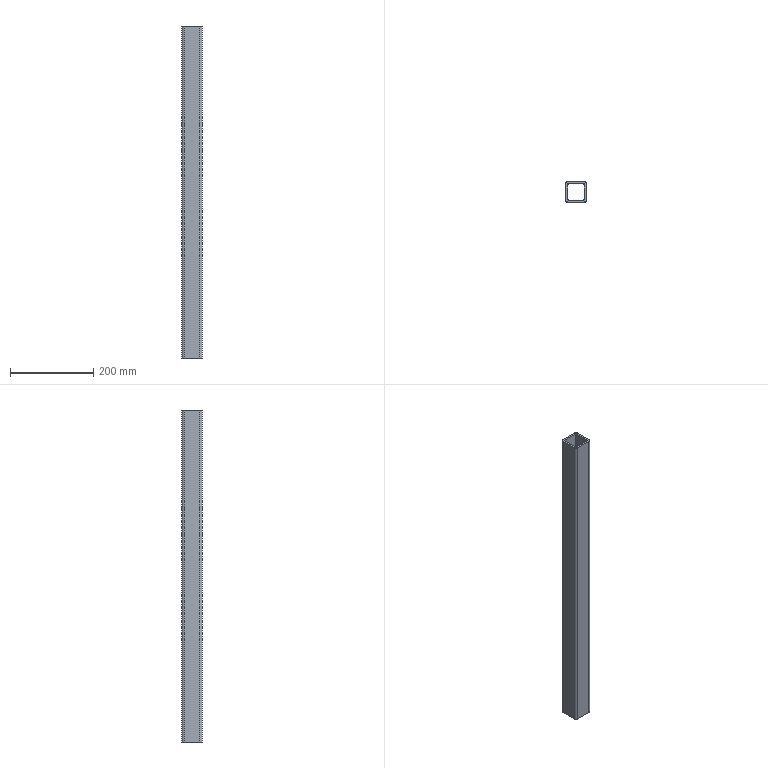Part | SolidWorks | features Extrusion 1 | 1 solid | 18 faces | box 50 x 50 x 800 mm | volume 695965 mm3 | plane 10 | cylinder 8 | commonest cylinder face diameters 2 x4 12 x4
STEP:
#1=CARTESIAN_POINT('',(0.,6.,800.));
#2=VERTEX_POINT('',#1);
#3=CARTESIAN_POINT('',(6.,0.,800.));
#4=VERTEX_POINT('',#3);
#5=CARTESIAN_POINT('',(6.,6.,800.));
#6=DIRECTION('',(0.,0.,1.));
#7=DIRECTION('',(-1.,0.,0.));
#8=AXIS2_PLACEMENT_3D('',#5,#6,#7);
#9=CIRCLE('',#8,6.);
#10=EDGE_CURVE('',#2,#4,#9,.T.);
#11=ORIENTED_EDGE('',*,*,#10,.T.);
#12=CARTESIAN_POINT('',(44.,0.,800.));
#13=VERTEX_POINT('',#12);
#14=CARTESIAN_POINT('',(6.,0.,800.));
#15=DIRECTION('',(1.,0.,0.));
#16=VECTOR('',#15,1000.);
#17=LINE('',#14,#16);
#18=EDGE_CURVE('',#4,#13,#17,.T.);
#19=ORIENTED_EDGE('',*,*,#18,.T.);
#20=CARTESIAN_POINT('',(50.,6.,800.));
#21=VERTEX_POINT('',#20);
#22=CARTESIAN_POINT('',(44.,6.,800.));
#23=DIRECTION('',(0.,0.,1.));
#24=DIRECTION('',(1.,0.,0.));
#25=AXIS2_PLACEMENT_3D('',#22,#23,#24);
#26=CIRCLE('',#25,6.);
#27=EDGE_CURVE('',#13,#21,#26,.T.);
#28=ORIENTED_EDGE('',*,*,#27,.T.);
#29=CARTESIAN_POINT('',(50.,44.,800.));
#30=VERTEX_POINT('',#29);
#31=CARTESIAN_POINT('',(50.,6.,800.));
#32=DIRECTION('',(0.,1.,0.));
#33=VECTOR('',#32,1000.);
#34=LINE('',#31,#33);
#35=EDGE_CURVE('',#21,#30,#34,.T.);
#36=ORIENTED_EDGE('',*,*,#35,.T.);
#37=CARTESIAN_POINT('',(44.,50.,800.));
#38=VERTEX_POINT('',#37);
#39=CARTESIAN_POINT('',(44.,44.,800.));
#40=DIRECTION('',(0.,0.,1.));
#41=DIRECTION('',(-1.,0.,0.));
#42=AXIS2_PLACEMENT_3D('',#39,#40,#41);
#43=CIRCLE('',#42,6.);
#44=EDGE_CURVE('',#30,#38,#43,.T.);
#45=ORIENTED_EDGE('',*,*,#44,.T.);
#46=CARTESIAN_POINT('',(6.,50.,800.));
#47=VERTEX_POINT('',#46);
#48=CARTESIAN_POINT('',(6.,50.,800.));
#49=DIRECTION('',(-1.,0.,0.));
#50=VECTOR('',#49,1000.);
#51=LINE('',#48,#50);
#52=EDGE_CURVE('',#38,#47,#51,.T.);
#53=ORIENTED_EDGE('',*,*,#52,.T.);
#54=CARTESIAN_POINT('',(0.,44.,800.));
#55=VERTEX_POINT('',#54);
#56=CARTESIAN_POINT('',(6.,44.,800.));
#57=DIRECTION('',(0.,0.,1.));
#58=DIRECTION('',(-1.,0.,0.));
#59=AXIS2_PLACEMENT_3D('',#56,#57,#58);
#60=CIRCLE('',#59,6.);
#61=EDGE_CURVE('',#47,#55,#60,.T.);
#62=ORIENTED_EDGE('',*,*,#61,.T.);
#63=CARTESIAN_POINT('',(0.,6.,800.));
#64=DIRECTION('',(0.,-1.,0.));
#65=VECTOR('',#64,1000.);
#66=LINE('',#63,#65);
#67=EDGE_CURVE('',#55,#2,#66,.T.);
#68=ORIENTED_EDGE('',*,*,#67,.T.);
#69=EDGE_LOOP('',(#11,#19,#28,#36,#45,#53,#62,#68));
#70=FACE_OUTER_BOUND('',#69,.T.);
#71=CARTESIAN_POINT('',(6.,45.,800.));
#72=VERTEX_POINT('',#71);
#73=CARTESIAN_POINT('',(5.,44.,800.));
#74=VERTEX_POINT('',#73);
#75=CARTESIAN_POINT('',(6.,44.,800.));
#76=DIRECTION('',(0.,0.,1.));
#77=DIRECTION('',(-1.,0.,0.));
#78=AXIS2_PLACEMENT_3D('',#75,#76,#77);
#79=CIRCLE('',#78,1.);
#80=EDGE_CURVE('',#72,#74,#79,.T.);
#81=ORIENTED_EDGE('',*,*,#80,.F.);
#82=CARTESIAN_POINT('',(44.,45.,800.));
#83=VERTEX_POINT('',#82);
#84=CARTESIAN_POINT('',(6.,45.,800.));
#85=DIRECTION('',(-1.,0.,0.));
#86=VECTOR('',#85,1000.);
#87=LINE('',#84,#86);
#88=EDGE_CURVE('',#83,#72,#87,.T.);
#89=ORIENTED_EDGE('',*,*,#88,.F.);
#90=CARTESIAN_POINT('',(45.,44.,800.));
#91=VERTEX_POINT('',#90);
#92=CARTESIAN_POINT('',(44.,44.,800.));
#93=DIRECTION('',(0.,0.,1.));
#94=DIRECTION('',(-1.,0.,0.));
#95=AXIS2_PLACEMENT_3D('',#92,#93,#94);
#96=CIRCLE('',#95,1.);
#97=EDGE_CURVE('',#91,#83,#96,.T.);
#98=ORIENTED_EDGE('',*,*,#97,.F.);
#99=CARTESIAN_POINT('',(45.,6.,800.));
#100=VERTEX_POINT('',#99);
#101=CARTESIAN_POINT('',(45.,6.,800.));
#102=DIRECTION('',(0.,1.,0.));
#103=VECTOR('',#102,1000.);
#104=LINE('',#101,#103);
#105=EDGE_CURVE('',#100,#91,#104,.T.);
#106=ORIENTED_EDGE('',*,*,#105,.F.);
#107=CARTESIAN_POINT('',(44.,5.,800.));
#108=VERTEX_POINT('',#107);
#109=CARTESIAN_POINT('',(44.,6.,800.));
#110=DIRECTION('',(0.,0.,1.));
#111=DIRECTION('',(1.,0.,0.));
#112=AXIS2_PLACEMENT_3D('',#109,#110,#111);
#113=CIRCLE('',#112,1.);
#114=EDGE_CURVE('',#108,#100,#113,.T.);
#115=ORIENTED_EDGE('',*,*,#114,.F.);
#116=CARTESIAN_POINT('',(6.,5.,800.));
#117=VERTEX_POINT('',#116);
#118=CARTESIAN_POINT('',(6.,5.,800.));
#119=DIRECTION('',(1.,0.,0.));
#120=VECTOR('',#119,1000.);
#121=LINE('',#118,#120);
#122=EDGE_CURVE('',#117,#108,#121,.T.);
#123=ORIENTED_EDGE('',*,*,#122,.F.);
#124=CARTESIAN_POINT('',(5.,6.,800.));
#125=VERTEX_POINT('',#124);
#126=CARTESIAN_POINT('',(6.,6.,800.));
#127=DIRECTION('',(0.,0.,1.));
#128=DIRECTION('',(-1.,0.,0.));
#129=AXIS2_PLACEMENT_3D('',#126,#127,#128);
#130=CIRCLE('',#129,1.);
#131=EDGE_CURVE('',#125,#117,#130,.T.);
#132=ORIENTED_EDGE('',*,*,#131,.F.);
#133=CARTESIAN_POINT('',(5.,6.,800.));
#134=DIRECTION('',(0.,-1.,0.));
#135=VECTOR('',#134,1000.);
#136=LINE('',#133,#135);
#137=EDGE_CURVE('',#74,#125,#136,.T.);
#138=ORIENTED_EDGE('',*,*,#137,.F.);
#139=EDGE_LOOP('',(#81,#89,#98,#106,#115,#123,#132,#138));
#140=FACE_BOUND('',#139,.T.);
#141=CARTESIAN_POINT('',(6.,6.,800.));
#142=DIRECTION('',(0.,0.,-1.));
#143=DIRECTION('',(-1.,0.,0.));
#144=AXIS2_PLACEMENT_3D('',#141,#142,#143);
#145=PLANE('',#144);
#146=ADVANCED_FACE('',(#70,#140),#145,.F.);
#147=CARTESIAN_POINT('',(0.,6.,0.));
#148=VERTEX_POINT('',#147);
#149=CARTESIAN_POINT('',(6.,0.,0.));
#150=VERTEX_POINT('',#149);
#151=CARTESIAN_POINT('',(6.,6.,0.));
#152=DIRECTION('',(0.,0.,1.));
#153=DIRECTION('',(-1.,0.,0.));
#154=AXIS2_PLACEMENT_3D('',#151,#152,#153);
#155=CIRCLE('',#154,6.);
#156=EDGE_CURVE('',#148,#150,#155,.T.);
#157=ORIENTED_EDGE('',*,*,#156,.F.);
#158=CARTESIAN_POINT('',(0.,44.,0.));
#159=VERTEX_POINT('',#158);
#160=CARTESIAN_POINT('',(0.,6.,0.));
#161=DIRECTION('',(0.,-1.,0.));
#162=VECTOR('',#161,1000.);
#163=LINE('',#160,#162);
#164=EDGE_CURVE('',#159,#148,#163,.T.);
#165=ORIENTED_EDGE('',*,*,#164,.F.);
#166=CARTESIAN_POINT('',(6.,50.,0.));
#167=VERTEX_POINT('',#166);
#168=CARTESIAN_POINT('',(6.,44.,0.));
#169=DIRECTION('',(0.,0.,1.));
#170=DIRECTION('',(-1.,0.,0.));
#171=AXIS2_PLACEMENT_3D('',#168,#169,#170);
#172=CIRCLE('',#171,6.);
#173=EDGE_CURVE('',#167,#159,#172,.T.);
#174=ORIENTED_EDGE('',*,*,#173,.F.);
#175=CARTESIAN_POINT('',(44.,50.,0.));
#176=VERTEX_POINT('',#175);
#177=CARTESIAN_POINT('',(6.,50.,0.));
#178=DIRECTION('',(-1.,0.,0.));
#179=VECTOR('',#178,1000.);
#180=LINE('',#177,#179);
#181=EDGE_CURVE('',#176,#167,#180,.T.);
#182=ORIENTED_EDGE('',*,*,#181,.F.);
#183=CARTESIAN_POINT('',(50.,44.,0.));
#184=VERTEX_POINT('',#183);
#185=CARTESIAN_POINT('',(44.,44.,0.));
#186=DIRECTION('',(0.,0.,1.));
#187=DIRECTION('',(-1.,0.,0.));
#188=AXIS2_PLACEMENT_3D('',#185,#186,#187);
#189=CIRCLE('',#188,6.);
#190=EDGE_CURVE('',#184,#176,#189,.T.);
#191=ORIENTED_EDGE('',*,*,#190,.F.);
#192=CARTESIAN_POINT('',(50.,6.,0.));
#193=VERTEX_POINT('',#192);
#194=CARTESIAN_POINT('',(50.,6.,0.));
#195=DIRECTION('',(0.,1.,0.));
#196=VECTOR('',#195,1000.);
#197=LINE('',#194,#196);
#198=EDGE_CURVE('',#193,#184,#197,.T.);
#199=ORIENTED_EDGE('',*,*,#198,.F.);
#200=CARTESIAN_POINT('',(44.,0.,0.));
#201=VERTEX_POINT('',#200);
#202=CARTESIAN_POINT('',(44.,6.,0.));
#203=DIRECTION('',(0.,0.,1.));
#204=DIRECTION('',(1.,0.,0.));
#205=AXIS2_PLACEMENT_3D('',#202,#203,#204);
#206=CIRCLE('',#205,6.);
#207=EDGE_CURVE('',#201,#193,#206,.T.);
#208=ORIENTED_EDGE('',*,*,#207,.F.);
#209=CARTESIAN_POINT('',(6.,0.,0.));
#210=DIRECTION('',(1.,0.,0.));
#211=VECTOR('',#210,1000.);
#212=LINE('',#209,#211);
#213=EDGE_CURVE('',#150,#201,#212,.T.);
#214=ORIENTED_EDGE('',*,*,#213,.F.);
#215=EDGE_LOOP('',(#157,#165,#174,#182,#191,#199,#208,#214));
#216=FACE_OUTER_BOUND('',#215,.T.);
#217=CARTESIAN_POINT('',(44.,45.,0.));
#218=VERTEX_POINT('',#217);
#219=CARTESIAN_POINT('',(6.,45.,0.));
#220=VERTEX_POINT('',#219);
#221=CARTESIAN_POINT('',(6.,45.,0.));
#222=DIRECTION('',(-1.,0.,0.));
#223=VECTOR('',#222,1000.);
#224=LINE('',#221,#223);
#225=EDGE_CURVE('',#218,#220,#224,.T.);
#226=ORIENTED_EDGE('',*,*,#225,.T.);
#227=CARTESIAN_POINT('',(5.,44.,0.));
#228=VERTEX_POINT('',#227);
#229=CARTESIAN_POINT('',(6.,44.,0.));
#230=DIRECTION('',(0.,0.,1.));
#231=DIRECTION('',(-1.,0.,0.));
#232=AXIS2_PLACEMENT_3D('',#229,#230,#231);
#233=CIRCLE('',#232,1.);
#234=EDGE_CURVE('',#220,#228,#233,.T.);
#235=ORIENTED_EDGE('',*,*,#234,.T.);
#236=CARTESIAN_POINT('',(5.,6.,0.));
#237=VERTEX_POINT('',#236);
#238=CARTESIAN_POINT('',(5.,6.,0.));
#239=DIRECTION('',(0.,-1.,0.));
#240=VECTOR('',#239,1000.);
#241=LINE('',#238,#240);
#242=EDGE_CURVE('',#228,#237,#241,.T.);
#243=ORIENTED_EDGE('',*,*,#242,.T.);
#244=CARTESIAN_POINT('',(6.,5.,0.));
#245=VERTEX_POINT('',#244);
#246=CARTESIAN_POINT('',(6.,6.,0.));
#247=DIRECTION('',(0.,0.,1.));
#248=DIRECTION('',(-1.,0.,0.));
#249=AXIS2_PLACEMENT_3D('',#246,#247,#248);
#250=CIRCLE('',#249,1.);
#251=EDGE_CURVE('',#237,#245,#250,.T.);
#252=ORIENTED_EDGE('',*,*,#251,.T.);
#253=CARTESIAN_POINT('',(44.,5.,0.));
#254=VERTEX_POINT('',#253);
#255=CARTESIAN_POINT('',(6.,5.,0.));
#256=DIRECTION('',(1.,0.,0.));
#257=VECTOR('',#256,1000.);
#258=LINE('',#255,#257);
#259=EDGE_CURVE('',#245,#254,#258,.T.);
#260=ORIENTED_EDGE('',*,*,#259,.T.);
#261=CARTESIAN_POINT('',(45.,6.,0.));
#262=VERTEX_POINT('',#261);
#263=CARTESIAN_POINT('',(44.,6.,0.));
#264=DIRECTION('',(0.,0.,1.));
#265=DIRECTION('',(1.,0.,0.));
#266=AXIS2_PLACEMENT_3D('',#263,#264,#265);
#267=CIRCLE('',#266,1.);
#268=EDGE_CURVE('',#254,#262,#267,.T.);
#269=ORIENTED_EDGE('',*,*,#268,.T.);
#270=CARTESIAN_POINT('',(45.,44.,0.));
#271=VERTEX_POINT('',#270);
#272=CARTESIAN_POINT('',(45.,6.,0.));
#273=DIRECTION('',(0.,1.,0.));
#274=VECTOR('',#273,1000.);
#275=LINE('',#272,#274);
#276=EDGE_CURVE('',#262,#271,#275,.T.);
#277=ORIENTED_EDGE('',*,*,#276,.T.);
#278=CARTESIAN_POINT('',(44.,44.,0.));
#279=DIRECTION('',(0.,0.,1.));
#280=DIRECTION('',(-1.,0.,0.));
#281=AXIS2_PLACEMENT_3D('',#278,#279,#280);
#282=CIRCLE('',#281,1.);
#283=EDGE_CURVE('',#271,#218,#282,.T.);
#284=ORIENTED_EDGE('',*,*,#283,.T.);
#285=EDGE_LOOP('',(#226,#235,#243,#252,#260,#269,#277,#284));
#286=FACE_BOUND('',#285,.T.);
#287=CARTESIAN_POINT('',(6.,6.,0.));
#288=DIRECTION('',(0.,0.,-1.));
#289=DIRECTION('',(-1.,0.,0.));
#290=AXIS2_PLACEMENT_3D('',#287,#288,#289);
#291=PLANE('',#290);
#292=ADVANCED_FACE('',(#216,#286),#291,.T.);
#293=ORIENTED_EDGE('',*,*,#156,.T.);
#294=CARTESIAN_POINT('',(6.,0.,800.));
#295=DIRECTION('',(0.,0.,-1.));
#296=VECTOR('',#295,1000.);
#297=LINE('',#294,#296);
#298=EDGE_CURVE('',#4,#150,#297,.T.);
#299=ORIENTED_EDGE('',*,*,#298,.F.);
#300=ORIENTED_EDGE('',*,*,#10,.F.);
#301=CARTESIAN_POINT('',(0.,6.,800.));
#302=DIRECTION('',(0.,0.,-1.));
#303=VECTOR('',#302,1000.);
#304=LINE('',#301,#303);
#305=EDGE_CURVE('',#2,#148,#304,.T.);
#306=ORIENTED_EDGE('',*,*,#305,.T.);
#307=EDGE_LOOP('',(#293,#299,#300,#306));
#308=FACE_OUTER_BOUND('',#307,.T.);
#309=CARTESIAN_POINT('',(6.,6.,800.));
#310=DIRECTION('',(0.,0.,-1.));
#311=DIRECTION('',(-1.,0.,0.));
#312=AXIS2_PLACEMENT_3D('',#309,#310,#311);
#313=CYLINDRICAL_SURFACE('',#312,6.);
#314=ADVANCED_FACE('',(#308),#313,.T.);
#315=ORIENTED_EDGE('',*,*,#213,.T.);
#316=CARTESIAN_POINT('',(44.,0.,800.));
#317=DIRECTION('',(0.,0.,-1.));
#318=VECTOR('',#317,1000.);
#319=LINE('',#316,#318);
#320=EDGE_CURVE('',#13,#201,#319,.T.);
#321=ORIENTED_EDGE('',*,*,#320,.F.);
#322=ORIENTED_EDGE('',*,*,#18,.F.);
#323=ORIENTED_EDGE('',*,*,#298,.T.);
#324=EDGE_LOOP('',(#315,#321,#322,#323));
#325=FACE_OUTER_BOUND('',#324,.T.);
#326=CARTESIAN_POINT('',(6.,0.,800.));
#327=DIRECTION('',(0.,1.,0.));
#328=DIRECTION('',(0.,0.,1.));
#329=AXIS2_PLACEMENT_3D('',#326,#327,#328);
#330=PLANE('',#329);
#331=ADVANCED_FACE('',(#325),#330,.F.);
#332=ORIENTED_EDGE('',*,*,#207,.T.);
#333=CARTESIAN_POINT('',(50.,6.,800.));
#334=DIRECTION('',(0.,0.,-1.));
#335=VECTOR('',#334,1000.);
#336=LINE('',#333,#335);
#337=EDGE_CURVE('',#21,#193,#336,.T.);
#338=ORIENTED_EDGE('',*,*,#337,.F.);
#339=ORIENTED_EDGE('',*,*,#27,.F.);
#340=ORIENTED_EDGE('',*,*,#320,.T.);
#341=EDGE_LOOP('',(#332,#338,#339,#340));
#342=FACE_OUTER_BOUND('',#341,.T.);
#343=CARTESIAN_POINT('',(44.,6.,800.));
#344=DIRECTION('',(0.,0.,-1.));
#345=DIRECTION('',(-1.,0.,0.));
#346=AXIS2_PLACEMENT_3D('',#343,#344,#345);
#347=CYLINDRICAL_SURFACE('',#346,6.);
#348=ADVANCED_FACE('',(#342),#347,.T.);
#349=ORIENTED_EDGE('',*,*,#198,.T.);
#350=CARTESIAN_POINT('',(50.,44.,800.));
#351=DIRECTION('',(0.,0.,-1.));
#352=VECTOR('',#351,1000.);
#353=LINE('',#350,#352);
#354=EDGE_CURVE('',#30,#184,#353,.T.);
#355=ORIENTED_EDGE('',*,*,#354,.F.);
#356=ORIENTED_EDGE('',*,*,#35,.F.);
#357=ORIENTED_EDGE('',*,*,#337,.T.);
#358=EDGE_LOOP('',(#349,#355,#356,#357));
#359=FACE_OUTER_BOUND('',#358,.T.);
#360=CARTESIAN_POINT('',(50.,6.,800.));
#361=DIRECTION('',(-1.,0.,0.));
#362=DIRECTION('',(0.,0.,1.));
#363=AXIS2_PLACEMENT_3D('',#360,#361,#362);
#364=PLANE('',#363);
#365=ADVANCED_FACE('',(#359),#364,.F.);
#366=ORIENTED_EDGE('',*,*,#190,.T.);
#367=CARTESIAN_POINT('',(44.,50.,800.));
#368=DIRECTION('',(0.,0.,-1.));
#369=VECTOR('',#368,1000.);
#370=LINE('',#367,#369);
#371=EDGE_CURVE('',#38,#176,#370,.T.);
#372=ORIENTED_EDGE('',*,*,#371,.F.);
#373=ORIENTED_EDGE('',*,*,#44,.F.);
#374=ORIENTED_EDGE('',*,*,#354,.T.);
#375=EDGE_LOOP('',(#366,#372,#373,#374));
#376=FACE_OUTER_BOUND('',#375,.T.);
#377=CARTESIAN_POINT('',(44.,44.,800.));
#378=DIRECTION('',(0.,0.,-1.));
#379=DIRECTION('',(-1.,0.,0.));
#380=AXIS2_PLACEMENT_3D('',#377,#378,#379);
#381=CYLINDRICAL_SURFACE('',#380,6.);
#382=ADVANCED_FACE('',(#376),#381,.T.);
#383=ORIENTED_EDGE('',*,*,#181,.T.);
#384=CARTESIAN_POINT('',(6.,50.,800.));
#385=DIRECTION('',(0.,0.,-1.));
#386=VECTOR('',#385,1000.);
#387=LINE('',#384,#386);
#388=EDGE_CURVE('',#47,#167,#387,.T.);
#389=ORIENTED_EDGE('',*,*,#388,.F.);
#390=ORIENTED_EDGE('',*,*,#52,.F.);
#391=ORIENTED_EDGE('',*,*,#371,.T.);
#392=EDGE_LOOP('',(#383,#389,#390,#391));
#393=FACE_OUTER_BOUND('',#392,.T.);
#394=CARTESIAN_POINT('',(6.,50.,800.));
#395=DIRECTION('',(0.,-1.,0.));
#396=DIRECTION('',(0.,0.,-1.));
#397=AXIS2_PLACEMENT_3D('',#394,#395,#396);
#398=PLANE('',#397);
#399=ADVANCED_FACE('',(#393),#398,.F.);
#400=ORIENTED_EDGE('',*,*,#173,.T.);
#401=CARTESIAN_POINT('',(0.,44.,800.));
#402=DIRECTION('',(0.,0.,-1.));
#403=VECTOR('',#402,1000.);
#404=LINE('',#401,#403);
#405=EDGE_CURVE('',#55,#159,#404,.T.);
#406=ORIENTED_EDGE('',*,*,#405,.F.);
#407=ORIENTED_EDGE('',*,*,#61,.F.);
#408=ORIENTED_EDGE('',*,*,#388,.T.);
#409=EDGE_LOOP('',(#400,#406,#407,#408));
#410=FACE_OUTER_BOUND('',#409,.T.);
#411=CARTESIAN_POINT('',(6.,44.,800.));
#412=DIRECTION('',(0.,0.,-1.));
#413=DIRECTION('',(-1.,0.,0.));
#414=AXIS2_PLACEMENT_3D('',#411,#412,#413);
#415=CYLINDRICAL_SURFACE('',#414,6.);
#416=ADVANCED_FACE('',(#410),#415,.T.);
#417=ORIENTED_EDGE('',*,*,#164,.T.);
#418=ORIENTED_EDGE('',*,*,#305,.F.);
#419=ORIENTED_EDGE('',*,*,#67,.F.);
#420=ORIENTED_EDGE('',*,*,#405,.T.);
#421=EDGE_LOOP('',(#417,#418,#419,#420));
#422=FACE_OUTER_BOUND('',#421,.T.);
#423=CARTESIAN_POINT('',(0.,6.,800.));
#424=DIRECTION('',(1.,0.,0.));
#425=DIRECTION('',(0.,0.,-1.));
#426=AXIS2_PLACEMENT_3D('',#423,#424,#425);
#427=PLANE('',#426);
#428=ADVANCED_FACE('',(#422),#427,.F.);
#429=ORIENTED_EDGE('',*,*,#234,.F.);
#430=CARTESIAN_POINT('',(6.,45.,800.));
#431=DIRECTION('',(0.,0.,-1.));
#432=VECTOR('',#431,1000.);
#433=LINE('',#430,#432);
#434=EDGE_CURVE('',#72,#220,#433,.T.);
#435=ORIENTED_EDGE('',*,*,#434,.F.);
#436=ORIENTED_EDGE('',*,*,#80,.T.);
#437=CARTESIAN_POINT('',(5.,44.,800.));
#438=DIRECTION('',(0.,0.,-1.));
#439=VECTOR('',#438,1000.);
#440=LINE('',#437,#439);
#441=EDGE_CURVE('',#74,#228,#440,.T.);
#442=ORIENTED_EDGE('',*,*,#441,.T.);
#443=EDGE_LOOP('',(#429,#435,#436,#442));
#444=FACE_OUTER_BOUND('',#443,.T.);
#445=CARTESIAN_POINT('',(6.,44.,800.));
#446=DIRECTION('',(0.,0.,-1.));
#447=DIRECTION('',(-1.,0.,0.));
#448=AXIS2_PLACEMENT_3D('',#445,#446,#447);
#449=CYLINDRICAL_SURFACE('',#448,1.);
#450=ADVANCED_FACE('',(#444),#449,.F.);
#451=ORIENTED_EDGE('',*,*,#242,.F.);
#452=ORIENTED_EDGE('',*,*,#441,.F.);
#453=ORIENTED_EDGE('',*,*,#137,.T.);
#454=CARTESIAN_POINT('',(5.,6.,800.));
#455=DIRECTION('',(0.,0.,-1.));
#456=VECTOR('',#455,1000.);
#457=LINE('',#454,#456);
#458=EDGE_CURVE('',#125,#237,#457,.T.);
#459=ORIENTED_EDGE('',*,*,#458,.T.);
#460=EDGE_LOOP('',(#451,#452,#453,#459));
#461=FACE_OUTER_BOUND('',#460,.T.);
#462=CARTESIAN_POINT('',(5.,6.,800.));
#463=DIRECTION('',(1.,0.,0.));
#464=DIRECTION('',(0.,1.,0.));
#465=AXIS2_PLACEMENT_3D('',#462,#463,#464);
#466=PLANE('',#465);
#467=ADVANCED_FACE('',(#461),#466,.T.);
#468=ORIENTED_EDGE('',*,*,#251,.F.);
#469=ORIENTED_EDGE('',*,*,#458,.F.);
#470=ORIENTED_EDGE('',*,*,#131,.T.);
#471=CARTESIAN_POINT('',(6.,5.,800.));
#472=DIRECTION('',(0.,0.,-1.));
#473=VECTOR('',#472,1000.);
#474=LINE('',#471,#473);
#475=EDGE_CURVE('',#117,#245,#474,.T.);
#476=ORIENTED_EDGE('',*,*,#475,.T.);
#477=EDGE_LOOP('',(#468,#469,#470,#476));
#478=FACE_OUTER_BOUND('',#477,.T.);
#479=CARTESIAN_POINT('',(6.,6.,800.));
#480=DIRECTION('',(0.,0.,-1.));
#481=DIRECTION('',(-1.,0.,0.));
#482=AXIS2_PLACEMENT_3D('',#479,#480,#481);
#483=CYLINDRICAL_SURFACE('',#482,1.);
#484=ADVANCED_FACE('',(#478),#483,.F.);
#485=ORIENTED_EDGE('',*,*,#259,.F.);
#486=ORIENTED_EDGE('',*,*,#475,.F.);
#487=ORIENTED_EDGE('',*,*,#122,.T.);
#488=CARTESIAN_POINT('',(44.,5.,800.));
#489=DIRECTION('',(0.,0.,-1.));
#490=VECTOR('',#489,1000.);
#491=LINE('',#488,#490);
#492=EDGE_CURVE('',#108,#254,#491,.T.);
#493=ORIENTED_EDGE('',*,*,#492,.T.);
#494=EDGE_LOOP('',(#485,#486,#487,#493));
#495=FACE_OUTER_BOUND('',#494,.T.);
#496=CARTESIAN_POINT('',(6.,5.,800.));
#497=DIRECTION('',(0.,1.,0.));
#498=DIRECTION('',(-1.,0.,0.));
#499=AXIS2_PLACEMENT_3D('',#496,#497,#498);
#500=PLANE('',#499);
#501=ADVANCED_FACE('',(#495),#500,.T.);
#502=ORIENTED_EDGE('',*,*,#268,.F.);
#503=ORIENTED_EDGE('',*,*,#492,.F.);
#504=ORIENTED_EDGE('',*,*,#114,.T.);
#505=CARTESIAN_POINT('',(45.,6.,800.));
#506=DIRECTION('',(0.,0.,-1.));
#507=VECTOR('',#506,1000.);
#508=LINE('',#505,#507);
#509=EDGE_CURVE('',#100,#262,#508,.T.);
#510=ORIENTED_EDGE('',*,*,#509,.T.);
#511=EDGE_LOOP('',(#502,#503,#504,#510));
#512=FACE_OUTER_BOUND('',#511,.T.);
#513=CARTESIAN_POINT('',(44.,6.,800.));
#514=DIRECTION('',(0.,0.,-1.));
#515=DIRECTION('',(-1.,0.,0.));
#516=AXIS2_PLACEMENT_3D('',#513,#514,#515);
#517=CYLINDRICAL_SURFACE('',#516,1.);
#518=ADVANCED_FACE('',(#512),#517,.F.);
#519=ORIENTED_EDGE('',*,*,#276,.F.);
#520=ORIENTED_EDGE('',*,*,#509,.F.);
#521=ORIENTED_EDGE('',*,*,#105,.T.);
#522=CARTESIAN_POINT('',(45.,44.,800.));
#523=DIRECTION('',(0.,0.,-1.));
#524=VECTOR('',#523,1000.);
#525=LINE('',#522,#524);
#526=EDGE_CURVE('',#91,#271,#525,.T.);
#527=ORIENTED_EDGE('',*,*,#526,.T.);
#528=EDGE_LOOP('',(#519,#520,#521,#527));
#529=FACE_OUTER_BOUND('',#528,.T.);
#530=CARTESIAN_POINT('',(45.,6.,800.));
#531=DIRECTION('',(-1.,0.,0.));
#532=DIRECTION('',(0.,0.,1.));
#533=AXIS2_PLACEMENT_3D('',#530,#531,#532);
#534=PLANE('',#533);
#535=ADVANCED_FACE('',(#529),#534,.T.);
#536=ORIENTED_EDGE('',*,*,#283,.F.);
#537=ORIENTED_EDGE('',*,*,#526,.F.);
#538=ORIENTED_EDGE('',*,*,#97,.T.);
#539=CARTESIAN_POINT('',(44.,45.,800.));
#540=DIRECTION('',(0.,0.,-1.));
#541=VECTOR('',#540,1000.);
#542=LINE('',#539,#541);
#543=EDGE_CURVE('',#83,#218,#542,.T.);
#544=ORIENTED_EDGE('',*,*,#543,.T.);
#545=EDGE_LOOP('',(#536,#537,#538,#544));
#546=FACE_OUTER_BOUND('',#545,.T.);
#547=CARTESIAN_POINT('',(44.,44.,800.));
#548=DIRECTION('',(0.,0.,-1.));
#549=DIRECTION('',(-1.,0.,0.));
#550=AXIS2_PLACEMENT_3D('',#547,#548,#549);
#551=CYLINDRICAL_SURFACE('',#550,1.);
#552=ADVANCED_FACE('',(#546),#551,.F.);
#553=ORIENTED_EDGE('',*,*,#225,.F.);
#554=ORIENTED_EDGE('',*,*,#543,.F.);
#555=ORIENTED_EDGE('',*,*,#88,.T.);
#556=ORIENTED_EDGE('',*,*,#434,.T.);
#557=EDGE_LOOP('',(#553,#554,#555,#556));
#558=FACE_OUTER_BOUND('',#557,.T.);
#559=CARTESIAN_POINT('',(6.,45.,800.));
#560=DIRECTION('',(0.,-1.,0.));
#561=DIRECTION('',(0.,0.,-1.));
#562=AXIS2_PLACEMENT_3D('',#559,#560,#561);
#563=PLANE('',#562);
#564=ADVANCED_FACE('',(#558),#563,.T.);
#565=CLOSED_SHELL('',(#146,#292,#314,#331,#348,#365,#382,#399,#416,#428,#450,#467,#484,#501,#518,#535,#552,#564));
#566=MANIFOLD_SOLID_BREP('',#565);
#567=CARTESIAN_POINT('',(0.,0.,0.));
#568=DIRECTION('',(0.,0.,1.));
#569=DIRECTION('',(1.,0.,0.));
#570=AXIS2_PLACEMENT_3D('',#567,#568,#569);
#571=(LENGTH_UNIT()NAMED_UNIT(*)SI_UNIT(.MILLI.,.METRE.));
#572=UNCERTAINTY_MEASURE_WITH_UNIT(LENGTH_MEASURE(0.00001),#571,'','');
#573=(NAMED_UNIT(*)PLANE_ANGLE_UNIT()SI_UNIT($,.RADIAN.));
#574=(NAMED_UNIT(*)SI_UNIT($,.STERADIAN.)SOLID_ANGLE_UNIT());
#575=(GEOMETRIC_REPRESENTATION_CONTEXT(3)GLOBAL_UNCERTAINTY_ASSIGNED_CONTEXT((#572))GLOBAL_UNIT_ASSIGNED_CONTEXT((#571,#573,#574))REPRESENTATION_CONTEXT('',''));
#576=ADVANCED_BREP_SHAPE_REPRESENTATION('',(#566,#570),#575);